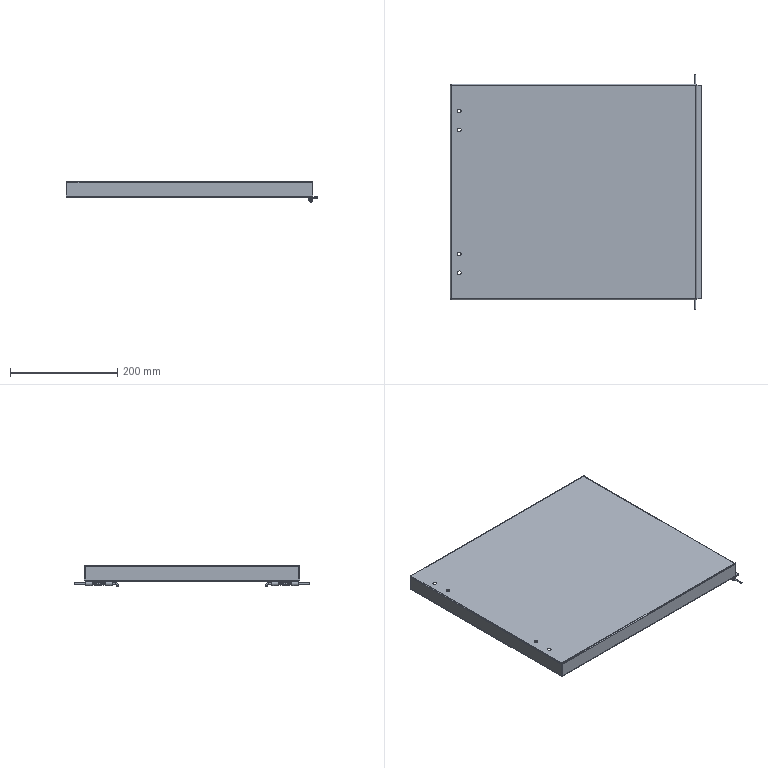Part | 5 solids | 145 faces | box 469.8 x 438.127 x 41 mm | volume 304650 mm3 | plane 76 | cylinder 51 | spline 14 | torus 4 | commonest cylinder face diameters 7 x11 1.473 x8 3 x8 3.6 x8 3.873 x8 7.6 x8